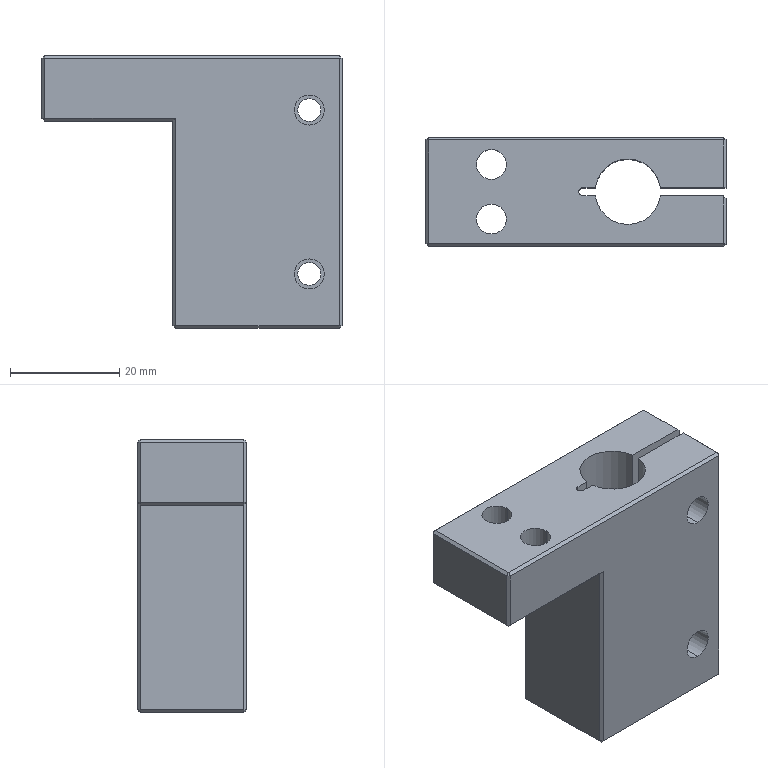Part | STEP file | ND25021-01-JDKM-35-TL | 1 solid | 59 faces | box 55 x 20 x 50 mm | volume 28654 mm3 | plane 43 | cylinder 16 | commonest cylinder face diameters 5.5 x8 4.2 x4 1.5 x2 12 x2